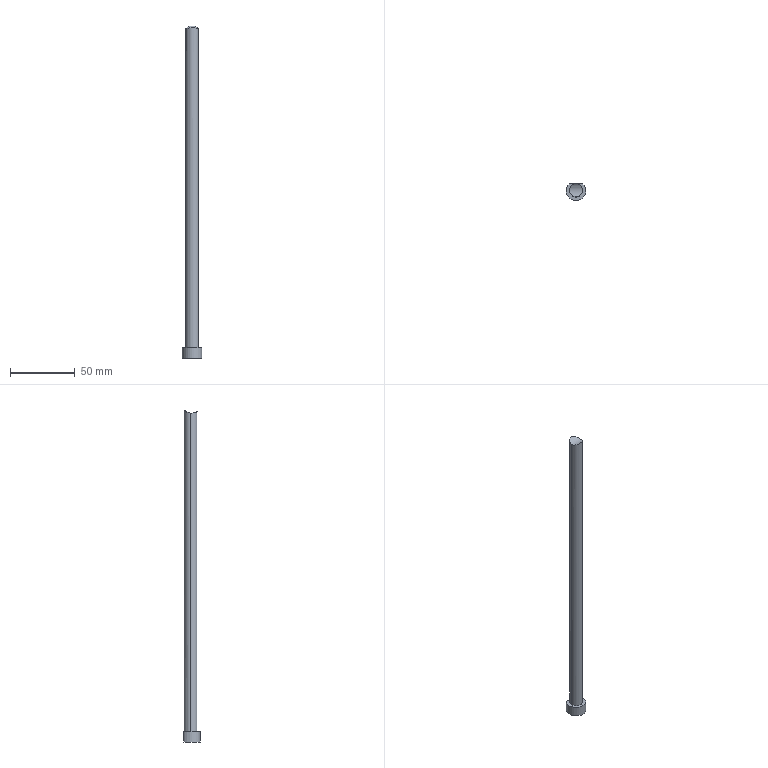Part | Creo | 1 solid | 7 faces | box 15 x 13 x 255.82 mm | volume 20611 mm3 | cylinder 4 | plane 3 | commonest cylinder face diameters 10 x2 15 x1 16.28 x1
STEP:
#1=CARTESIAN_POINT('',(0.,0.,0.));
#2=DIRECTION('',(0.,0.,1.));
#3=DIRECTION('',(1.,0.,0.));
#4=AXIS2_PLACEMENT_3D('',#1,#2,#3);
#5=CARTESIAN_POINT('',(10.408,11.708,-330.441));
#6=VERTEX_POINT('',#5);
#7=CARTESIAN_POINT('',(0.2097,11.708,-330.441));
#8=VERTEX_POINT('',#7);
#9=CARTESIAN_POINT('',(10.408,11.708,-330.441));
#10=DIRECTION('',(-1.,0.,0.));
#11=VECTOR('',#10,10.198);
#12=LINE('',#9,#11);
#13=EDGE_CURVE('',#6,#8,#12,.T.);
#14=ORIENTED_EDGE('',*,*,#13,.F.);
#15=CARTESIAN_POINT('',(5.309,6.208,-330.441));
#16=DIRECTION('',(0.,0.,-1.));
#17=DIRECTION('',(0.6799,0.7333,0.));
#18=AXIS2_PLACEMENT_3D('',#15,#16,#17);
#19=CIRCLE('',#18,7.5);
#20=EDGE_CURVE('',#6,#8,#19,.T.);
#21=ORIENTED_EDGE('',*,*,#20,.T.);
#22=EDGE_LOOP('',(#14,#21));
#23=FACE_OUTER_BOUND('',#22,.F.);
#24=CARTESIAN_POINT('',(0.3087,6.208,-330.441));
#25=VERTEX_POINT('',#24);
#26=CARTESIAN_POINT('',(10.309,6.208,-330.441));
#27=VERTEX_POINT('',#26);
#28=CARTESIAN_POINT('',(5.309,6.208,-330.441));
#29=DIRECTION('',(0.,0.,-1.));
#30=DIRECTION('',(-1.,0.,0.));
#31=AXIS2_PLACEMENT_3D('',#28,#29,#30);
#32=CIRCLE('',#31,5.);
#33=EDGE_CURVE('',#25,#27,#32,.T.);
#34=ORIENTED_EDGE('',*,*,#33,.F.);
#35=CARTESIAN_POINT('',(5.309,6.208,-330.441));
#36=DIRECTION('',(0.,0.,-1.));
#37=DIRECTION('',(1.,0.,0.));
#38=AXIS2_PLACEMENT_3D('',#35,#36,#37);
#39=CIRCLE('',#38,5.);
#40=EDGE_CURVE('',#27,#25,#39,.T.);
#41=ORIENTED_EDGE('',*,*,#40,.F.);
#42=EDGE_LOOP('',(#34,#41));
#43=FACE_BOUND('',#42,.F.);
#44=CARTESIAN_POINT('',(5.309,6.208,-330.441));
#45=DIRECTION('',(0.,0.,-1.));
#46=DIRECTION('',(-1.,0.,0.));
#47=AXIS2_PLACEMENT_3D('',#44,#45,#46);
#48=PLANE('',#47);
#49=ADVANCED_FACE('',(#23,#43),#48,.F.);
#50=CARTESIAN_POINT('',(10.309,6.208,-84.987));
#51=VERTEX_POINT('',#50);
#52=CARTESIAN_POINT('',(0.3089,6.208,-84.987));
#53=VERTEX_POINT('',#52);
#54=CARTESIAN_POINT('',(10.309,6.208,-84.987));
#55=CARTESIAN_POINT('',(10.309,6.61,-84.949));
#56=CARTESIAN_POINT('',(10.214,7.413,-84.813));
#57=CARTESIAN_POINT('',(9.756,8.616,-84.412));
#58=CARTESIAN_POINT('',(8.98,9.688,-83.854));
#59=CARTESIAN_POINT('',(7.965,10.503,-83.271));
#60=CARTESIAN_POINT('',(6.921,10.983,-82.845));
#61=CARTESIAN_POINT('',(5.849,11.219,-82.61));
#62=CARTESIAN_POINT('',(4.746,11.216,-82.614));
#63=CARTESIAN_POINT('',(3.684,10.979,-82.849));
#64=CARTESIAN_POINT('',(2.644,10.498,-83.275));
#65=CARTESIAN_POINT('',(1.631,9.681,-83.859));
#66=CARTESIAN_POINT('',(0.8584,8.61,-84.414));
#67=CARTESIAN_POINT('',(0.4003,7.402,-84.816));
#68=CARTESIAN_POINT('',(0.3089,6.606,-84.949));
#69=CARTESIAN_POINT('',(0.3089,6.208,-84.987));
#70=B_SPLINE_CURVE_WITH_KNOTS('',3,(#54,#55,#56,#57,#58,#59,#60,#61,#62,#63,#64,#65,#66,#67,#68,#69),.UNSPECIFIED.,.F.,.F.,(4,1,1,1,1,1,1,1,1,1,1,1,1,4),(0.,0.07692,0.1538,0.2308,0.3077,0.3846,0.4615,0.5385,0.6154,0.6923,0.7692,0.8462,0.9231,1.),.UNSPECIFIED.);
#71=EDGE_CURVE('',#51,#53,#70,.T.);
#72=ORIENTED_EDGE('',*,*,#71,.T.);
#73=CARTESIAN_POINT('',(0.3087,6.208,-330.441));
#74=DIRECTION('',(0.000000845,0.000000099,1.));
#75=VECTOR('',#74,245.454);
#76=LINE('',#73,#75);
#77=EDGE_CURVE('',#25,#53,#76,.T.);
#78=ORIENTED_EDGE('',*,*,#77,.F.);
#79=ORIENTED_EDGE('',*,*,#33,.T.);
#80=CARTESIAN_POINT('',(10.309,6.208,-330.441));
#81=DIRECTION('',(0.,0.,1.));
#82=VECTOR('',#81,245.454);
#83=LINE('',#80,#82);
#84=EDGE_CURVE('',#27,#51,#83,.T.);
#85=ORIENTED_EDGE('',*,*,#84,.T.);
#86=EDGE_LOOP('',(#72,#78,#79,#85));
#87=FACE_OUTER_BOUND('',#86,.F.);
#88=CARTESIAN_POINT('',(5.309,6.208,-653.441));
#89=DIRECTION('',(0.,0.,1.));
#90=DIRECTION('',(1.,0.,0.));
#91=AXIS2_PLACEMENT_3D('',#88,#89,#90);
#92=CYLINDRICAL_SURFACE('',#91,5.);
#93=ADVANCED_FACE('',(#87),#92,.T.);
#94=ORIENTED_EDGE('',*,*,#71,.F.);
#95=CARTESIAN_POINT('',(10.247,5.433,-85.022));
#96=VERTEX_POINT('',#95);
#97=CARTESIAN_POINT('',(10.247,5.433,-85.022));
#98=CARTESIAN_POINT('',(10.261,5.52,-85.022));
#99=CARTESIAN_POINT('',(10.285,5.693,-85.023));
#100=CARTESIAN_POINT('',(10.304,5.951,-85.009));
#101=CARTESIAN_POINT('',(10.309,6.123,-84.995));
#102=CARTESIAN_POINT('',(10.309,6.208,-84.987));
#103=B_SPLINE_CURVE_WITH_KNOTS('',3,(#97,#98,#99,#100,#101,#102),.UNSPECIFIED.,.F.,.F.,(4,1,1,4),(0.,0.3333,0.6667,1.),.UNSPECIFIED.);
#104=EDGE_CURVE('',#96,#51,#103,.T.);
#105=ORIENTED_EDGE('',*,*,#104,.F.);
#106=CARTESIAN_POINT('',(0.3718,5.433,-85.02));
#107=VERTEX_POINT('',#106);
#108=CARTESIAN_POINT('',(0.3718,5.433,-85.02));
#109=CARTESIAN_POINT('',(0.4354,5.028,-85.02));
#110=CARTESIAN_POINT('',(0.6531,4.245,-84.967));
#111=CARTESIAN_POINT('',(1.293,3.139,-84.718));
#112=CARTESIAN_POINT('',(2.193,2.228,-84.383));
#113=CARTESIAN_POINT('',(3.321,1.555,-84.049));
#114=CARTESIAN_POINT('',(4.645,1.189,-83.831));
#115=CARTESIAN_POINT('',(6.025,1.196,-83.835));
#116=CARTESIAN_POINT('',(7.349,1.578,-84.062));
#117=CARTESIAN_POINT('',(8.464,2.26,-84.397));
#118=CARTESIAN_POINT('',(9.349,3.174,-84.728));
#119=CARTESIAN_POINT('',(9.971,4.267,-84.968));
#120=CARTESIAN_POINT('',(10.185,5.037,-85.022));
#121=B_SPLINE_CURVE_WITH_KNOTS('',3,(#108,#109,#110,#111,#112,#113,#114,#115,#116,#117,#118,#119,#120,#95),.UNSPECIFIED.,.F.,.F.,(4,1,1,1,1,1,1,1,1,1,1,4),(0.,0.09091,0.1818,0.2727,0.3636,0.4545,0.5455,0.6364,0.7273,0.8182,0.9091,1.),.UNSPECIFIED.);
#122=EDGE_CURVE('',#107,#96,#121,.T.);
#123=ORIENTED_EDGE('',*,*,#122,.F.);
#124=CARTESIAN_POINT('',(0.3089,6.208,-84.987));
#125=CARTESIAN_POINT('',(0.3089,6.123,-84.995));
#126=CARTESIAN_POINT('',(0.3133,5.952,-85.009));
#127=CARTESIAN_POINT('',(0.3318,5.693,-85.023));
#128=CARTESIAN_POINT('',(0.3582,5.52,-85.02));
#129=B_SPLINE_CURVE_WITH_KNOTS('',3,(#124,#125,#126,#127,#128,#106),.UNSPECIFIED.,.F.,.F.,(4,1,1,4),(0.,0.3333,0.6667,1.),.UNSPECIFIED.);
#130=EDGE_CURVE('',#53,#107,#129,.T.);
#131=ORIENTED_EDGE('',*,*,#130,.F.);
#132=EDGE_LOOP('',(#94,#105,#123,#131));
#133=FACE_OUTER_BOUND('',#132,.F.);
#134=CARTESIAN_POINT('',(-4.387,5.433,-76.884));
#135=DIRECTION('',(1.,-0.000000007,0.000000135));
#136=DIRECTION('',(0.000000135,0.,-1.));
#137=AXIS2_PLACEMENT_3D('',#134,#135,#136);
#138=CYLINDRICAL_SURFACE('',#137,8.14);
#139=ADVANCED_FACE('',(#133),#138,.F.);
#140=ORIENTED_EDGE('',*,*,#130,.T.);
#141=ORIENTED_EDGE('',*,*,#122,.T.);
#142=ORIENTED_EDGE('',*,*,#104,.T.);
#143=ORIENTED_EDGE('',*,*,#84,.F.);
#144=ORIENTED_EDGE('',*,*,#40,.T.);
#145=ORIENTED_EDGE('',*,*,#77,.T.);
#146=EDGE_LOOP('',(#140,#141,#142,#143,#144,#145));
#147=FACE_OUTER_BOUND('',#146,.F.);
#148=CARTESIAN_POINT('',(5.309,6.208,-653.441));
#149=DIRECTION('',(0.,0.,1.));
#150=DIRECTION('',(1.,0.,0.));
#151=AXIS2_PLACEMENT_3D('',#148,#149,#150);
#152=CYLINDRICAL_SURFACE('',#151,5.);
#153=ADVANCED_FACE('',(#147),#152,.T.);
#154=CARTESIAN_POINT('',(0.2097,11.708,-338.441));
#155=VERTEX_POINT('',#154);
#156=CARTESIAN_POINT('',(0.2097,11.708,-330.441));
#157=DIRECTION('',(0.,0.,-1.));
#158=VECTOR('',#157,8.);
#159=LINE('',#156,#158);
#160=EDGE_CURVE('',#8,#155,#159,.T.);
#161=ORIENTED_EDGE('',*,*,#160,.T.);
#162=CARTESIAN_POINT('',(10.408,11.708,-338.441));
#163=VERTEX_POINT('',#162);
#164=CARTESIAN_POINT('',(10.408,11.708,-338.441));
#165=DIRECTION('',(-1.,0.,0.));
#166=VECTOR('',#165,10.198);
#167=LINE('',#164,#166);
#168=EDGE_CURVE('',#163,#155,#167,.T.);
#169=ORIENTED_EDGE('',*,*,#168,.F.);
#170=CARTESIAN_POINT('',(10.408,11.708,-338.441));
#171=DIRECTION('',(0.,0.,1.));
#172=VECTOR('',#171,8.);
#173=LINE('',#170,#172);
#174=EDGE_CURVE('',#163,#6,#173,.T.);
#175=ORIENTED_EDGE('',*,*,#174,.T.);
#176=ORIENTED_EDGE('',*,*,#13,.T.);
#177=EDGE_LOOP('',(#161,#169,#175,#176));
#178=FACE_OUTER_BOUND('',#177,.F.);
#179=CARTESIAN_POINT('',(5.309,11.708,-338.441));
#180=DIRECTION('',(0.,1.,0.));
#181=DIRECTION('',(0.,0.,1.));
#182=AXIS2_PLACEMENT_3D('',#179,#180,#181);
#183=PLANE('',#182);
#184=ADVANCED_FACE('',(#178),#183,.T.);
#185=CARTESIAN_POINT('',(5.309,6.208,-338.441));
#186=DIRECTION('',(0.,0.,1.));
#187=DIRECTION('',(-0.6799,0.7333,0.));
#188=AXIS2_PLACEMENT_3D('',#185,#186,#187);
#189=CIRCLE('',#188,7.5);
#190=EDGE_CURVE('',#155,#163,#189,.T.);
#191=ORIENTED_EDGE('',*,*,#190,.F.);
#192=ORIENTED_EDGE('',*,*,#160,.F.);
#193=ORIENTED_EDGE('',*,*,#20,.F.);
#194=ORIENTED_EDGE('',*,*,#174,.F.);
#195=EDGE_LOOP('',(#191,#192,#193,#194));
#196=FACE_OUTER_BOUND('',#195,.F.);
#197=CARTESIAN_POINT('',(5.309,6.208,-330.441));
#198=DIRECTION('',(0.,0.,-1.));
#199=DIRECTION('',(-1.,0.,0.));
#200=AXIS2_PLACEMENT_3D('',#197,#198,#199);
#201=CYLINDRICAL_SURFACE('',#200,7.5);
#202=ADVANCED_FACE('',(#196),#201,.T.);
#203=ORIENTED_EDGE('',*,*,#190,.T.);
#204=ORIENTED_EDGE('',*,*,#168,.T.);
#205=EDGE_LOOP('',(#203,#204));
#206=FACE_OUTER_BOUND('',#205,.F.);
#207=CARTESIAN_POINT('',(5.309,6.208,-338.441));
#208=DIRECTION('',(0.,0.,-1.));
#209=DIRECTION('',(-1.,0.,0.));
#210=AXIS2_PLACEMENT_3D('',#207,#208,#209);
#211=PLANE('',#210);
#212=ADVANCED_FACE('',(#206),#211,.T.);
#213=CLOSED_SHELL('',(#49,#93,#139,#153,#184,#202,#212));
#214=MANIFOLD_SOLID_BREP('',#213);
#215=(LENGTH_UNIT()NAMED_UNIT(*)SI_UNIT(.MILLI.,.METRE.));
#216=UNCERTAINTY_MEASURE_WITH_UNIT(LENGTH_MEASURE(0.02566),#215,'','');
#217=(NAMED_UNIT(*)PLANE_ANGLE_UNIT()SI_UNIT($,.RADIAN.));
#218=PLANE_ANGLE_MEASURE_WITH_UNIT(PLANE_ANGLE_MEASURE(0.01745),#217);
#219=(CONVERSION_BASED_UNIT('DEGREE',#218)NAMED_UNIT(*)PLANE_ANGLE_UNIT());
#220=(NAMED_UNIT(*)SI_UNIT($,.STERADIAN.)SOLID_ANGLE_UNIT());
#221=(GEOMETRIC_REPRESENTATION_CONTEXT(3)GLOBAL_UNCERTAINTY_ASSIGNED_CONTEXT((#216))GLOBAL_UNIT_ASSIGNED_CONTEXT((#215,#219,#220))REPRESENTATION_CONTEXT('',''));
#222=ADVANCED_BREP_SHAPE_REPRESENTATION('',(#4,#214),#221);